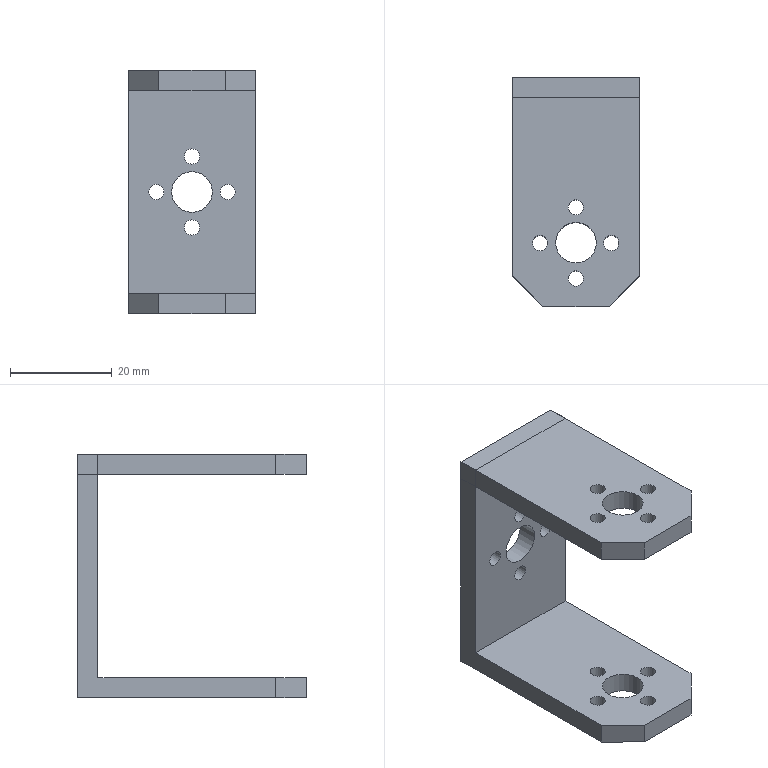Part | NX | features DATUM_CSYS 4, EXTRUDE 3, MOVE_FACE 3, SKETCH 3, EXTRACT_BODY 2, EXTRACT_FACE 2, EXTRACT_STRING 2, Instance Feature 1, Mirror Feature 1, Pattern Geometry 1 | 2 solids | 33 faces | box 25 x 45 x 48 mm | volume 12170 mm3 | plane 18 | cylinder 15 | commonest cylinder face diameters 3 x12 8 x3
STEP:
#1=CARTESIAN_POINT('',(-12.454,5.071,-2.));
#2=VERTEX_POINT('',#1);
#3=CARTESIAN_POINT('',(-12.454,44.071,-2.));
#4=VERTEX_POINT('',#3);
#5=CARTESIAN_POINT('',(-12.454,24.071,-2.));
#6=DIRECTION('',(0.,1.,0.));
#7=VECTOR('',#6,1000.);
#8=LINE('',#5,#7);
#9=EDGE_CURVE('',#2,#4,#8,.T.);
#10=ORIENTED_EDGE('',*,*,#9,.F.);
#11=CARTESIAN_POINT('',(-12.454,5.071,2.));
#12=VERTEX_POINT('',#11);
#13=CARTESIAN_POINT('',(-12.454,5.071,8.));
#14=DIRECTION('',(0.,0.,-1.));
#15=VECTOR('',#14,1000.);
#16=LINE('',#13,#15);
#17=EDGE_CURVE('',#12,#2,#16,.T.);
#18=ORIENTED_EDGE('',*,*,#17,.F.);
#19=CARTESIAN_POINT('',(-12.454,44.071,2.));
#20=VERTEX_POINT('',#19);
#21=CARTESIAN_POINT('',(-12.454,5.071,2.));
#22=DIRECTION('',(0.,1.,0.));
#23=VECTOR('',#22,1000.);
#24=LINE('',#21,#23);
#25=EDGE_CURVE('',#12,#20,#24,.T.);
#26=ORIENTED_EDGE('',*,*,#25,.T.);
#27=CARTESIAN_POINT('',(-12.454,44.071,8.));
#28=DIRECTION('',(0.,0.,-1.));
#29=VECTOR('',#28,1000.);
#30=LINE('',#27,#29);
#31=EDGE_CURVE('',#20,#4,#30,.T.);
#32=ORIENTED_EDGE('',*,*,#31,.T.);
#33=EDGE_LOOP('',(#10,#18,#26,#32));
#34=FACE_BOUND('',#33,.T.);
#35=CARTESIAN_POINT('',(-12.454,24.071,8.));
#36=DIRECTION('',(-1.,0.,0.));
#37=DIRECTION('',(0.,-1.,0.));
#38=AXIS2_PLACEMENT_3D('',#35,#36,#37);
#39=PLANE('',#38);
#40=ADVANCED_FACE('',(#34),#39,.T.);
#41=CARTESIAN_POINT('',(12.546,44.071,-2.));
#42=VERTEX_POINT('',#41);
#43=CARTESIAN_POINT('',(-12.454,44.071,-2.));
#44=DIRECTION('',(1.,0.,0.));
#45=VECTOR('',#44,1000.);
#46=LINE('',#43,#45);
#47=EDGE_CURVE('',#4,#42,#46,.T.);
#48=ORIENTED_EDGE('',*,*,#47,.F.);
#49=ORIENTED_EDGE('',*,*,#31,.F.);
#50=CARTESIAN_POINT('',(12.546,44.071,2.));
#51=VERTEX_POINT('',#50);
#52=CARTESIAN_POINT('',(-12.454,44.071,2.));
#53=DIRECTION('',(1.,0.,0.));
#54=VECTOR('',#53,1000.);
#55=LINE('',#52,#54);
#56=EDGE_CURVE('',#20,#51,#55,.T.);
#57=ORIENTED_EDGE('',*,*,#56,.T.);
#58=CARTESIAN_POINT('',(12.546,44.071,8.));
#59=DIRECTION('',(0.,0.,-1.));
#60=VECTOR('',#59,1000.);
#61=LINE('',#58,#60);
#62=EDGE_CURVE('',#51,#42,#61,.T.);
#63=ORIENTED_EDGE('',*,*,#62,.T.);
#64=EDGE_LOOP('',(#48,#49,#57,#63));
#65=FACE_BOUND('',#64,.T.);
#66=CARTESIAN_POINT('',(-12.454,44.071,8.));
#67=DIRECTION('',(0.,1.,0.));
#68=DIRECTION('',(0.,0.,1.));
#69=AXIS2_PLACEMENT_3D('',#66,#67,#68);
#70=PLANE('',#69);
#71=ADVANCED_FACE('',(#65),#70,.T.);
#72=CARTESIAN_POINT('',(12.546,5.071,-2.));
#73=VERTEX_POINT('',#72);
#74=CARTESIAN_POINT('',(12.546,24.071,-2.));
#75=DIRECTION('',(0.,-1.,0.));
#76=VECTOR('',#75,1000.);
#77=LINE('',#74,#76);
#78=EDGE_CURVE('',#42,#73,#77,.T.);
#79=ORIENTED_EDGE('',*,*,#78,.F.);
#80=ORIENTED_EDGE('',*,*,#62,.F.);
#81=CARTESIAN_POINT('',(12.546,5.071,2.));
#82=VERTEX_POINT('',#81);
#83=CARTESIAN_POINT('',(12.546,44.071,2.));
#84=DIRECTION('',(0.,-1.,0.));
#85=VECTOR('',#84,1000.);
#86=LINE('',#83,#85);
#87=EDGE_CURVE('',#51,#82,#86,.T.);
#88=ORIENTED_EDGE('',*,*,#87,.T.);
#89=CARTESIAN_POINT('',(12.546,5.071,8.));
#90=DIRECTION('',(0.,0.,-1.));
#91=VECTOR('',#90,1000.);
#92=LINE('',#89,#91);
#93=EDGE_CURVE('',#82,#73,#92,.T.);
#94=ORIENTED_EDGE('',*,*,#93,.T.);
#95=EDGE_LOOP('',(#79,#80,#88,#94));
#96=FACE_BOUND('',#95,.T.);
#97=CARTESIAN_POINT('',(12.546,24.071,8.));
#98=DIRECTION('',(1.,0.,0.));
#99=DIRECTION('',(0.,1.,0.));
#100=AXIS2_PLACEMENT_3D('',#97,#98,#99);
#101=PLANE('',#100);
#102=ADVANCED_FACE('',(#96),#101,.T.);
#103=CARTESIAN_POINT('',(6.546,-0.9291,-2.));
#104=VERTEX_POINT('',#103);
#105=CARTESIAN_POINT('',(12.546,5.071,-2.));
#106=DIRECTION('',(-0.7071,-0.7071,0.));
#107=VECTOR('',#106,1000.);
#108=LINE('',#105,#107);
#109=EDGE_CURVE('',#73,#104,#108,.T.);
#110=ORIENTED_EDGE('',*,*,#109,.F.);
#111=ORIENTED_EDGE('',*,*,#93,.F.);
#112=CARTESIAN_POINT('',(6.546,-0.9291,2.));
#113=VERTEX_POINT('',#112);
#114=CARTESIAN_POINT('',(12.546,5.071,2.));
#115=DIRECTION('',(-0.7071,-0.7071,0.));
#116=VECTOR('',#115,1000.);
#117=LINE('',#114,#116);
#118=EDGE_CURVE('',#82,#113,#117,.T.);
#119=ORIENTED_EDGE('',*,*,#118,.T.);
#120=CARTESIAN_POINT('',(6.546,-0.9291,8.));
#121=DIRECTION('',(0.,0.,-1.));
#122=VECTOR('',#121,1000.);
#123=LINE('',#120,#122);
#124=EDGE_CURVE('',#113,#104,#123,.T.);
#125=ORIENTED_EDGE('',*,*,#124,.T.);
#126=EDGE_LOOP('',(#110,#111,#119,#125));
#127=FACE_BOUND('',#126,.T.);
#128=CARTESIAN_POINT('',(12.546,5.071,8.));
#129=DIRECTION('',(0.7071,-0.7071,0.));
#130=DIRECTION('',(0.7071,0.7071,0.));
#131=AXIS2_PLACEMENT_3D('',#128,#129,#130);
#132=PLANE('',#131);
#133=ADVANCED_FACE('',(#127),#132,.T.);
#134=CARTESIAN_POINT('',(-6.454,-0.9291,-2.));
#135=VERTEX_POINT('',#134);
#136=CARTESIAN_POINT('',(6.546,-0.9291,-2.));
#137=DIRECTION('',(-1.,0.,0.));
#138=VECTOR('',#137,1000.);
#139=LINE('',#136,#138);
#140=EDGE_CURVE('',#104,#135,#139,.T.);
#141=ORIENTED_EDGE('',*,*,#140,.F.);
#142=ORIENTED_EDGE('',*,*,#124,.F.);
#143=CARTESIAN_POINT('',(-6.454,-0.9291,2.));
#144=VERTEX_POINT('',#143);
#145=CARTESIAN_POINT('',(6.546,-0.9291,2.));
#146=DIRECTION('',(-1.,0.,0.));
#147=VECTOR('',#146,1000.);
#148=LINE('',#145,#147);
#149=EDGE_CURVE('',#113,#144,#148,.T.);
#150=ORIENTED_EDGE('',*,*,#149,.T.);
#151=CARTESIAN_POINT('',(-6.454,-0.9291,8.));
#152=DIRECTION('',(0.,0.,-1.));
#153=VECTOR('',#152,1000.);
#154=LINE('',#151,#153);
#155=EDGE_CURVE('',#144,#135,#154,.T.);
#156=ORIENTED_EDGE('',*,*,#155,.T.);
#157=EDGE_LOOP('',(#141,#142,#150,#156));
#158=FACE_BOUND('',#157,.T.);
#159=CARTESIAN_POINT('',(6.546,-0.9291,8.));
#160=DIRECTION('',(0.,-1.,0.));
#161=DIRECTION('',(0.,0.,-1.));
#162=AXIS2_PLACEMENT_3D('',#159,#160,#161);
#163=PLANE('',#162);
#164=ADVANCED_FACE('',(#158),#163,.T.);
#165=CARTESIAN_POINT('',(1.5,4.5,2.));
#166=VERTEX_POINT('',#165);
#167=CARTESIAN_POINT('',(0.,4.5,2.));
#168=DIRECTION('',(0.,0.,-1.));
#169=DIRECTION('',(1.,0.,0.));
#170=AXIS2_PLACEMENT_3D('',#167,#168,#169);
#171=CIRCLE('',#170,1.5);
#172=EDGE_CURVE('',#166,#166,#171,.T.);
#173=ORIENTED_EDGE('',*,*,#172,.F.);
#174=EDGE_LOOP('',(#173));
#175=FACE_BOUND('',#174,.T.);
#176=CARTESIAN_POINT('',(1.5,4.5,-2.));
#177=VERTEX_POINT('',#176);
#178=CARTESIAN_POINT('',(0.,4.5,-2.));
#179=DIRECTION('',(0.,0.,-1.));
#180=DIRECTION('',(1.,0.,0.));
#181=AXIS2_PLACEMENT_3D('',#178,#179,#180);
#182=CIRCLE('',#181,1.5);
#183=EDGE_CURVE('',#177,#177,#182,.T.);
#184=ORIENTED_EDGE('',*,*,#183,.T.);
#185=EDGE_LOOP('',(#184));
#186=FACE_BOUND('',#185,.T.);
#187=CARTESIAN_POINT('',(0.,4.5,8.));
#188=DIRECTION('',(0.,0.,-1.));
#189=DIRECTION('',(-1.,0.,0.));
#190=AXIS2_PLACEMENT_3D('',#187,#188,#189);
#191=CYLINDRICAL_SURFACE('',#190,1.5);
#192=ADVANCED_FACE('',(#175,#186),#191,.F.);
#193=CARTESIAN_POINT('',(-5.5,11.5,2.));
#194=VERTEX_POINT('',#193);
#195=CARTESIAN_POINT('',(-7.,11.5,2.));
#196=DIRECTION('',(0.,0.,-1.));
#197=DIRECTION('',(1.,0.,0.));
#198=AXIS2_PLACEMENT_3D('',#195,#196,#197);
#199=CIRCLE('',#198,1.5);
#200=EDGE_CURVE('',#194,#194,#199,.T.);
#201=ORIENTED_EDGE('',*,*,#200,.F.);
#202=EDGE_LOOP('',(#201));
#203=FACE_BOUND('',#202,.T.);
#204=CARTESIAN_POINT('',(-5.5,11.5,-2.));
#205=VERTEX_POINT('',#204);
#206=CARTESIAN_POINT('',(-7.,11.5,-2.));
#207=DIRECTION('',(0.,0.,-1.));
#208=DIRECTION('',(1.,0.,0.));
#209=AXIS2_PLACEMENT_3D('',#206,#207,#208);
#210=CIRCLE('',#209,1.5);
#211=EDGE_CURVE('',#205,#205,#210,.T.);
#212=ORIENTED_EDGE('',*,*,#211,.T.);
#213=EDGE_LOOP('',(#212));
#214=FACE_BOUND('',#213,.T.);
#215=CARTESIAN_POINT('',(-7.,11.5,8.));
#216=DIRECTION('',(0.,0.,-1.));
#217=DIRECTION('',(-1.,0.,0.));
#218=AXIS2_PLACEMENT_3D('',#215,#216,#217);
#219=CYLINDRICAL_SURFACE('',#218,1.5);
#220=ADVANCED_FACE('',(#203,#214),#219,.F.);
#221=CARTESIAN_POINT('',(4.046,11.571,2.));
#222=VERTEX_POINT('',#221);
#223=CARTESIAN_POINT('',(0.04628,11.571,2.));
#224=DIRECTION('',(0.,0.,-1.));
#225=DIRECTION('',(1.,0.,0.));
#226=AXIS2_PLACEMENT_3D('',#223,#224,#225);
#227=CIRCLE('',#226,4.);
#228=EDGE_CURVE('',#222,#222,#227,.T.);
#229=ORIENTED_EDGE('',*,*,#228,.F.);
#230=EDGE_LOOP('',(#229));
#231=FACE_BOUND('',#230,.T.);
#232=CARTESIAN_POINT('',(4.046,11.571,-2.));
#233=VERTEX_POINT('',#232);
#234=CARTESIAN_POINT('',(0.04628,11.571,-2.));
#235=DIRECTION('',(0.,0.,-1.));
#236=DIRECTION('',(1.,0.,0.));
#237=AXIS2_PLACEMENT_3D('',#234,#235,#236);
#238=CIRCLE('',#237,4.);
#239=EDGE_CURVE('',#233,#233,#238,.T.);
#240=ORIENTED_EDGE('',*,*,#239,.T.);
#241=EDGE_LOOP('',(#240));
#242=FACE_BOUND('',#241,.T.);
#243=CARTESIAN_POINT('',(0.04628,11.571,8.));
#244=DIRECTION('',(0.,0.,-1.));
#245=DIRECTION('',(-1.,0.,0.));
#246=AXIS2_PLACEMENT_3D('',#243,#244,#245);
#247=CYLINDRICAL_SURFACE('',#246,4.);
#248=ADVANCED_FACE('',(#231,#242),#247,.F.);
#249=CARTESIAN_POINT('',(1.5,18.5,2.));
#250=VERTEX_POINT('',#249);
#251=CARTESIAN_POINT('',(0.,18.5,2.));
#252=DIRECTION('',(0.,0.,-1.));
#253=DIRECTION('',(1.,0.,0.));
#254=AXIS2_PLACEMENT_3D('',#251,#252,#253);
#255=CIRCLE('',#254,1.5);
#256=EDGE_CURVE('',#250,#250,#255,.T.);
#257=ORIENTED_EDGE('',*,*,#256,.F.);
#258=EDGE_LOOP('',(#257));
#259=FACE_BOUND('',#258,.T.);
#260=CARTESIAN_POINT('',(1.5,18.5,-2.));
#261=VERTEX_POINT('',#260);
#262=CARTESIAN_POINT('',(0.,18.5,-2.));
#263=DIRECTION('',(0.,0.,-1.));
#264=DIRECTION('',(1.,0.,0.));
#265=AXIS2_PLACEMENT_3D('',#262,#263,#264);
#266=CIRCLE('',#265,1.5);
#267=EDGE_CURVE('',#261,#261,#266,.T.);
#268=ORIENTED_EDGE('',*,*,#267,.T.);
#269=EDGE_LOOP('',(#268));
#270=FACE_BOUND('',#269,.T.);
#271=CARTESIAN_POINT('',(0.,18.5,8.));
#272=DIRECTION('',(0.,0.,-1.));
#273=DIRECTION('',(-1.,0.,0.));
#274=AXIS2_PLACEMENT_3D('',#271,#272,#273);
#275=CYLINDRICAL_SURFACE('',#274,1.5);
#276=ADVANCED_FACE('',(#259,#270),#275,.F.);
#277=CARTESIAN_POINT('',(-6.454,-0.9291,-2.));
#278=DIRECTION('',(-0.7071,0.7071,0.));
#279=VECTOR('',#278,1000.);
#280=LINE('',#277,#279);
#281=EDGE_CURVE('',#135,#2,#280,.T.);
#282=ORIENTED_EDGE('',*,*,#281,.F.);
#283=ORIENTED_EDGE('',*,*,#155,.F.);
#284=CARTESIAN_POINT('',(-6.454,-0.9291,2.));
#285=DIRECTION('',(-0.7071,0.7071,0.));
#286=VECTOR('',#285,1000.);
#287=LINE('',#284,#286);
#288=EDGE_CURVE('',#144,#12,#287,.T.);
#289=ORIENTED_EDGE('',*,*,#288,.T.);
#290=ORIENTED_EDGE('',*,*,#17,.T.);
#291=EDGE_LOOP('',(#282,#283,#289,#290));
#292=FACE_BOUND('',#291,.T.);
#293=CARTESIAN_POINT('',(-6.454,-0.9291,8.));
#294=DIRECTION('',(-0.7071,-0.7071,0.));
#295=DIRECTION('',(0.7071,-0.7071,0.));
#296=AXIS2_PLACEMENT_3D('',#293,#294,#295);
#297=PLANE('',#296);
#298=ADVANCED_FACE('',(#292),#297,.T.);
#299=CARTESIAN_POINT('',(8.5,11.5,2.));
#300=VERTEX_POINT('',#299);
#301=CARTESIAN_POINT('',(7.,11.5,2.));
#302=DIRECTION('',(0.,0.,-1.));
#303=DIRECTION('',(1.,0.,0.));
#304=AXIS2_PLACEMENT_3D('',#301,#302,#303);
#305=CIRCLE('',#304,1.5);
#306=EDGE_CURVE('',#300,#300,#305,.T.);
#307=ORIENTED_EDGE('',*,*,#306,.F.);
#308=EDGE_LOOP('',(#307));
#309=FACE_BOUND('',#308,.T.);
#310=CARTESIAN_POINT('',(8.5,11.5,-2.));
#311=VERTEX_POINT('',#310);
#312=CARTESIAN_POINT('',(7.,11.5,-2.));
#313=DIRECTION('',(0.,0.,-1.));
#314=DIRECTION('',(1.,0.,0.));
#315=AXIS2_PLACEMENT_3D('',#312,#313,#314);
#316=CIRCLE('',#315,1.5);
#317=EDGE_CURVE('',#311,#311,#316,.T.);
#318=ORIENTED_EDGE('',*,*,#317,.T.);
#319=EDGE_LOOP('',(#318));
#320=FACE_BOUND('',#319,.T.);
#321=CARTESIAN_POINT('',(7.,11.5,8.));
#322=DIRECTION('',(0.,0.,-1.));
#323=DIRECTION('',(-1.,0.,0.));
#324=AXIS2_PLACEMENT_3D('',#321,#322,#323);
#325=CYLINDRICAL_SURFACE('',#324,1.5);
#326=ADVANCED_FACE('',(#309,#320),#325,.F.);
#327=ORIENTED_EDGE('',*,*,#25,.F.);
#328=ORIENTED_EDGE('',*,*,#288,.F.);
#329=ORIENTED_EDGE('',*,*,#149,.F.);
#330=ORIENTED_EDGE('',*,*,#118,.F.);
#331=ORIENTED_EDGE('',*,*,#87,.F.);
#332=ORIENTED_EDGE('',*,*,#56,.F.);
#333=EDGE_LOOP('',(#327,#328,#329,#330,#331,#332));
#334=FACE_BOUND('',#333,.T.);
#335=ORIENTED_EDGE('',*,*,#256,.T.);
#336=EDGE_LOOP('',(#335));
#337=FACE_BOUND('',#336,.T.);
#338=ORIENTED_EDGE('',*,*,#228,.T.);
#339=EDGE_LOOP('',(#338));
#340=FACE_BOUND('',#339,.T.);
#341=ORIENTED_EDGE('',*,*,#200,.T.);
#342=EDGE_LOOP('',(#341));
#343=FACE_BOUND('',#342,.T.);
#344=ORIENTED_EDGE('',*,*,#172,.T.);
#345=EDGE_LOOP('',(#344));
#346=FACE_BOUND('',#345,.T.);
#347=ORIENTED_EDGE('',*,*,#306,.T.);
#348=EDGE_LOOP('',(#347));
#349=FACE_BOUND('',#348,.T.);
#350=CARTESIAN_POINT('',(0.,18.5,2.));
#351=DIRECTION('',(0.,0.,-1.));
#352=DIRECTION('',(-1.,0.,0.));
#353=AXIS2_PLACEMENT_3D('',#350,#351,#352);
#354=PLANE('',#353);
#355=ADVANCED_FACE('',(#334,#337,#340,#343,#346,#349),#354,.F.);
#356=ORIENTED_EDGE('',*,*,#281,.T.);
#357=ORIENTED_EDGE('',*,*,#9,.T.);
#358=ORIENTED_EDGE('',*,*,#47,.T.);
#359=ORIENTED_EDGE('',*,*,#78,.T.);
#360=ORIENTED_EDGE('',*,*,#109,.T.);
#361=ORIENTED_EDGE('',*,*,#140,.T.);
#362=EDGE_LOOP('',(#356,#357,#358,#359,#360,#361));
#363=FACE_BOUND('',#362,.T.);
#364=ORIENTED_EDGE('',*,*,#267,.F.);
#365=EDGE_LOOP('',(#364));
#366=FACE_BOUND('',#365,.T.);
#367=ORIENTED_EDGE('',*,*,#239,.F.);
#368=EDGE_LOOP('',(#367));
#369=FACE_BOUND('',#368,.T.);
#370=ORIENTED_EDGE('',*,*,#211,.F.);
#371=EDGE_LOOP('',(#370));
#372=FACE_BOUND('',#371,.T.);
#373=ORIENTED_EDGE('',*,*,#183,.F.);
#374=EDGE_LOOP('',(#373));
#375=FACE_BOUND('',#374,.T.);
#376=ORIENTED_EDGE('',*,*,#317,.F.);
#377=EDGE_LOOP('',(#376));
#378=FACE_BOUND('',#377,.T.);
#379=CARTESIAN_POINT('',(0.,18.5,-2.));
#380=DIRECTION('',(0.,0.,-1.));
#381=DIRECTION('',(-1.,0.,0.));
#382=AXIS2_PLACEMENT_3D('',#379,#380,#381);
#383=PLANE('',#382);
#384=ADVANCED_FACE('',(#363,#366,#369,#372,#375,#378),#383,.T.);
#385=CLOSED_SHELL('',(#40,#71,#102,#133,#164,#192,#220,#248,#276,#298,#326,#355,#384));
#386=MANIFOLD_SOLID_BREP('',#385);
#387=CARTESIAN_POINT('',(8.5,11.5,-42.));
#388=VERTEX_POINT('',#387);
#389=CARTESIAN_POINT('',(7.,11.5,-42.));
#390=DIRECTION('',(0.,0.,-1.));
#391=DIRECTION('',(1.,0.,0.));
#392=AXIS2_PLACEMENT_3D('',#389,#390,#391);
#393=CIRCLE('',#392,1.5);
#394=EDGE_CURVE('',#388,#388,#393,.T.);
#395=ORIENTED_EDGE('',*,*,#394,.T.);
#396=EDGE_LOOP('',(#395));
#397=FACE_BOUND('',#396,.T.);
#398=CARTESIAN_POINT('',(1.5,4.5,-42.));
#399=VERTEX_POINT('',#398);
#400=CARTESIAN_POINT('',(0.,4.5,-42.));
#401=DIRECTION('',(0.,0.,-1.));
#402=DIRECTION('',(1.,0.,0.));
#403=AXIS2_PLACEMENT_3D('',#400,#401,#402);
#404=CIRCLE('',#403,1.5);
#405=EDGE_CURVE('',#399,#399,#404,.T.);
#406=ORIENTED_EDGE('',*,*,#405,.T.);
#407=EDGE_LOOP('',(#406));
#408=FACE_BOUND('',#407,.T.);
#409=CARTESIAN_POINT('',(-5.5,11.5,-42.));
#410=VERTEX_POINT('',#409);
#411=CARTESIAN_POINT('',(-7.,11.5,-42.));
#412=DIRECTION('',(0.,0.,-1.));
#413=DIRECTION('',(1.,0.,0.));
#414=AXIS2_PLACEMENT_3D('',#411,#412,#413);
#415=CIRCLE('',#414,1.5);
#416=EDGE_CURVE('',#410,#410,#415,.T.);
#417=ORIENTED_EDGE('',*,*,#416,.T.);
#418=EDGE_LOOP('',(#417));
#419=FACE_BOUND('',#418,.T.);
#420=CARTESIAN_POINT('',(4.046,11.571,-42.));
#421=VERTEX_POINT('',#420);
#422=CARTESIAN_POINT('',(0.04628,11.571,-42.));
#423=DIRECTION('',(0.,0.,-1.));
#424=DIRECTION('',(1.,0.,0.));
#425=AXIS2_PLACEMENT_3D('',#422,#423,#424);
#426=CIRCLE('',#425,4.);
#427=EDGE_CURVE('',#421,#421,#426,.T.);
#428=ORIENTED_EDGE('',*,*,#427,.T.);
#429=EDGE_LOOP('',(#428));
#430=FACE_BOUND('',#429,.T.);
#431=CARTESIAN_POINT('',(1.5,18.5,-42.));
#432=VERTEX_POINT('',#431);
#433=CARTESIAN_POINT('',(0.,18.5,-42.));
#434=DIRECTION('',(0.,0.,-1.));
#435=DIRECTION('',(1.,0.,0.));
#436=AXIS2_PLACEMENT_3D('',#433,#434,#435);
#437=CIRCLE('',#436,1.5);
#438=EDGE_CURVE('',#432,#432,#437,.T.);
#439=ORIENTED_EDGE('',*,*,#438,.T.);
#440=EDGE_LOOP('',(#439));
#441=FACE_BOUND('',#440,.T.);
#442=CARTESIAN_POINT('',(12.546,40.071,-42.));
#443=VERTEX_POINT('',#442);
#444=CARTESIAN_POINT('',(-12.454,40.071,-42.));
#445=VERTEX_POINT('',#444);
#446=CARTESIAN_POINT('',(0.,40.071,-42.));
#447=DIRECTION('',(1.,0.,0.));
#448=VECTOR('',#447,1000.);
#449=LINE('',#446,#448);
#450=EDGE_CURVE('',#443,#445,#449,.F.);
#451=ORIENTED_EDGE('',*,*,#450,.T.);
#452=CARTESIAN_POINT('',(-12.454,5.071,-42.));
#453=VERTEX_POINT('',#452);
#454=CARTESIAN_POINT('',(-12.454,24.071,-42.));
#455=DIRECTION('',(0.,1.,0.));
#456=VECTOR('',#455,1000.);
#457=LINE('',#454,#456);
#458=EDGE_CURVE('',#453,#445,#457,.T.);
#459=ORIENTED_EDGE('',*,*,#458,.F.);
#460=CARTESIAN_POINT('',(-6.454,-0.9291,-42.));
#461=VERTEX_POINT('',#460);
#462=CARTESIAN_POINT('',(-6.454,-0.9291,-42.));
#463=DIRECTION('',(-0.7071,0.7071,0.));
#464=VECTOR('',#463,1000.);
#465=LINE('',#462,#464);
#466=EDGE_CURVE('',#461,#453,#465,.T.);
#467=ORIENTED_EDGE('',*,*,#466,.F.);
#468=CARTESIAN_POINT('',(6.546,-0.9291,-42.));
#469=VERTEX_POINT('',#468);
#470=CARTESIAN_POINT('',(6.546,-0.9291,-42.));
#471=DIRECTION('',(-1.,0.,0.));
#472=VECTOR('',#471,1000.);
#473=LINE('',#470,#472);
#474=EDGE_CURVE('',#469,#461,#473,.T.);
#475=ORIENTED_EDGE('',*,*,#474,.F.);
#476=CARTESIAN_POINT('',(12.546,5.071,-42.));
#477=VERTEX_POINT('',#476);
#478=CARTESIAN_POINT('',(12.546,5.071,-42.));
#479=DIRECTION('',(-0.7071,-0.7071,0.));
#480=VECTOR('',#479,1000.);
#481=LINE('',#478,#480);
#482=EDGE_CURVE('',#477,#469,#481,.T.);
#483=ORIENTED_EDGE('',*,*,#482,.F.);
#484=CARTESIAN_POINT('',(12.546,24.071,-42.));
#485=DIRECTION('',(0.,-1.,0.));
#486=VECTOR('',#485,1000.);
#487=LINE('',#484,#486);
#488=EDGE_CURVE('',#443,#477,#487,.T.);
#489=ORIENTED_EDGE('',*,*,#488,.F.);
#490=EDGE_LOOP('',(#451,#459,#467,#475,#483,#489));
#491=FACE_BOUND('',#490,.T.);
#492=CARTESIAN_POINT('',(0.,18.5,-42.));
#493=DIRECTION('',(0.,0.,-1.));
#494=DIRECTION('',(-1.,0.,0.));
#495=AXIS2_PLACEMENT_3D('',#492,#493,#494);
#496=PLANE('',#495);
#497=ADVANCED_FACE('',(#397,#408,#419,#430,#441,#491),#496,.F.);
#498=ORIENTED_EDGE('',*,*,#458,.T.);
#499=CARTESIAN_POINT('',(-12.454,40.071,2.));
#500=VERTEX_POINT('',#499);
#501=CARTESIAN_POINT('',(-12.454,40.071,4.));
#502=DIRECTION('',(0.,0.,-1.));
#503=VECTOR('',#502,1000.);
#504=LINE('',#501,#503);
#505=EDGE_CURVE('',#500,#445,#504,.T.);
#506=ORIENTED_EDGE('',*,*,#505,.F.);
#507=CARTESIAN_POINT('',(-12.454,44.071,2.));
#508=VERTEX_POINT('',#507);
#509=CARTESIAN_POINT('',(-12.454,40.071,2.));
#510=DIRECTION('',(0.,1.,0.));
#511=VECTOR('',#510,1000.);
#512=LINE('',#509,#511);
#513=EDGE_CURVE('',#500,#508,#512,.T.);
#514=ORIENTED_EDGE('',*,*,#513,.T.);
#515=CARTESIAN_POINT('',(-12.454,44.071,-46.));
#516=VERTEX_POINT('',#515);
#517=CARTESIAN_POINT('',(-12.454,44.071,-52.));
#518=DIRECTION('',(0.,0.,1.));
#519=VECTOR('',#518,1000.);
#520=LINE('',#517,#519);
#521=EDGE_CURVE('',#516,#508,#520,.T.);
#522=ORIENTED_EDGE('',*,*,#521,.F.);
#523=CARTESIAN_POINT('',(-12.454,5.071,-46.));
#524=VERTEX_POINT('',#523);
#525=CARTESIAN_POINT('',(-12.454,5.071,-46.));
#526=DIRECTION('',(0.,1.,0.));
#527=VECTOR('',#526,1000.);
#528=LINE('',#525,#527);
#529=EDGE_CURVE('',#524,#516,#528,.T.);
#530=ORIENTED_EDGE('',*,*,#529,.F.);
#531=CARTESIAN_POINT('',(-12.454,5.071,-52.));
#532=DIRECTION('',(0.,0.,1.));
#533=VECTOR('',#532,1000.);
#534=LINE('',#531,#533);
#535=EDGE_CURVE('',#524,#453,#534,.T.);
#536=ORIENTED_EDGE('',*,*,#535,.T.);
#537=EDGE_LOOP('',(#498,#506,#514,#522,#530,#536));
#538=FACE_BOUND('',#537,.T.);
#539=CARTESIAN_POINT('',(-12.454,24.071,-52.));
#540=DIRECTION('',(1.,0.,0.));
#541=DIRECTION('',(0.,1.,0.));
#542=AXIS2_PLACEMENT_3D('',#539,#540,#541);
#543=PLANE('',#542);
#544=ADVANCED_FACE('',(#538),#543,.F.);
#545=ORIENTED_EDGE('',*,*,#521,.T.);
#546=CARTESIAN_POINT('',(12.546,44.071,2.));
#547=VERTEX_POINT('',#546);
#548=CARTESIAN_POINT('',(12.546,44.071,2.));
#549=DIRECTION('',(-1.,0.,0.));
#550=VECTOR('',#549,1000.);
#551=LINE('',#548,#550);
#552=EDGE_CURVE('',#547,#508,#551,.T.);
#553=ORIENTED_EDGE('',*,*,#552,.F.);
#554=CARTESIAN_POINT('',(12.546,44.071,-46.));
#555=VERTEX_POINT('',#554);
#556=CARTESIAN_POINT('',(12.546,44.071,-52.));
#557=DIRECTION('',(0.,0.,1.));
#558=VECTOR('',#557,1000.);
#559=LINE('',#556,#558);
#560=EDGE_CURVE('',#555,#547,#559,.T.);
#561=ORIENTED_EDGE('',*,*,#560,.F.);
#562=CARTESIAN_POINT('',(-12.454,44.071,-46.));
#563=DIRECTION('',(1.,0.,0.));
#564=VECTOR('',#563,1000.);
#565=LINE('',#562,#564);
#566=EDGE_CURVE('',#516,#555,#565,.T.);
#567=ORIENTED_EDGE('',*,*,#566,.F.);
#568=EDGE_LOOP('',(#545,#553,#561,#567));
#569=FACE_BOUND('',#568,.T.);
#570=CARTESIAN_POINT('',(-6.954,44.071,-23.5));
#571=VERTEX_POINT('',#570);
#572=CARTESIAN_POINT('',(-6.954,44.071,-22.));
#573=DIRECTION('',(0.,1.,0.));
#574=DIRECTION('',(0.,0.,-1.));
#575=AXIS2_PLACEMENT_3D('',#572,#573,#574);
#576=CIRCLE('',#575,1.5);
#577=EDGE_CURVE('',#571,#571,#576,.T.);
#578=ORIENTED_EDGE('',*,*,#577,.F.);
#579=EDGE_LOOP('',(#578));
#580=FACE_BOUND('',#579,.T.);
#581=CARTESIAN_POINT('',(0.04628,44.071,-26.));
#582=VERTEX_POINT('',#581);
#583=CARTESIAN_POINT('',(0.04628,44.071,-22.));
#584=DIRECTION('',(0.,1.,0.));
#585=DIRECTION('',(0.,0.,-1.));
#586=AXIS2_PLACEMENT_3D('',#583,#584,#585);
#587=CIRCLE('',#586,4.);
#588=EDGE_CURVE('',#582,#582,#587,.T.);
#589=ORIENTED_EDGE('',*,*,#588,.F.);
#590=EDGE_LOOP('',(#589));
#591=FACE_BOUND('',#590,.T.);
#592=CARTESIAN_POINT('',(0.04628,44.071,-30.5));
#593=VERTEX_POINT('',#592);
#594=CARTESIAN_POINT('',(0.04628,44.071,-29.));
#595=DIRECTION('',(0.,1.,0.));
#596=DIRECTION('',(0.,0.,-1.));
#597=AXIS2_PLACEMENT_3D('',#594,#595,#596);
#598=CIRCLE('',#597,1.5);
#599=EDGE_CURVE('',#593,#593,#598,.T.);
#600=ORIENTED_EDGE('',*,*,#599,.F.);
#601=EDGE_LOOP('',(#600));
#602=FACE_BOUND('',#601,.T.);
#603=CARTESIAN_POINT('',(0.04628,44.071,-16.5));
#604=VERTEX_POINT('',#603);
#605=CARTESIAN_POINT('',(0.04628,44.071,-15.));
#606=DIRECTION('',(0.,1.,0.));
#607=DIRECTION('',(0.,0.,-1.));
#608=AXIS2_PLACEMENT_3D('',#605,#606,#607);
#609=CIRCLE('',#608,1.5);
#610=EDGE_CURVE('',#604,#604,#609,.T.);
#611=ORIENTED_EDGE('',*,*,#610,.F.);
#612=EDGE_LOOP('',(#611));
#613=FACE_BOUND('',#612,.T.);
#614=CARTESIAN_POINT('',(7.046,44.071,-23.5));
#615=VERTEX_POINT('',#614);
#616=CARTESIAN_POINT('',(7.046,44.071,-22.));
#617=DIRECTION('',(0.,1.,0.));
#618=DIRECTION('',(0.,0.,-1.));
#619=AXIS2_PLACEMENT_3D('',#616,#617,#618);
#620=CIRCLE('',#619,1.5);
#621=EDGE_CURVE('',#615,#615,#620,.T.);
#622=ORIENTED_EDGE('',*,*,#621,.F.);
#623=EDGE_LOOP('',(#622));
#624=FACE_BOUND('',#623,.T.);
#625=CARTESIAN_POINT('',(-12.454,44.071,-52.));
#626=DIRECTION('',(0.,-1.,0.));
#627=DIRECTION('',(0.,0.,-1.));
#628=AXIS2_PLACEMENT_3D('',#625,#626,#627);
#629=PLANE('',#628);
#630=ADVANCED_FACE('',(#569,#580,#591,#602,#613,#624),#629,.F.);
#631=CARTESIAN_POINT('',(12.546,5.071,-46.));
#632=VERTEX_POINT('',#631);
#633=CARTESIAN_POINT('',(12.546,5.071,-52.));
#634=DIRECTION('',(0.,0.,1.));
#635=VECTOR('',#634,1000.);
#636=LINE('',#633,#635);
#637=EDGE_CURVE('',#632,#477,#636,.T.);
#638=ORIENTED_EDGE('',*,*,#637,.F.);
#639=CARTESIAN_POINT('',(12.546,44.071,-46.));
#640=DIRECTION('',(0.,-1.,0.));
#641=VECTOR('',#640,1000.);
#642=LINE('',#639,#641);
#643=EDGE_CURVE('',#555,#632,#642,.T.);
#644=ORIENTED_EDGE('',*,*,#643,.F.);
#645=ORIENTED_EDGE('',*,*,#560,.T.);
#646=CARTESIAN_POINT('',(12.546,40.071,2.));
#647=VERTEX_POINT('',#646);
#648=CARTESIAN_POINT('',(12.546,40.071,2.));
#649=DIRECTION('',(0.,1.,0.));
#650=VECTOR('',#649,1000.);
#651=LINE('',#648,#650);
#652=EDGE_CURVE('',#647,#547,#651,.T.);
#653=ORIENTED_EDGE('',*,*,#652,.F.);
#654=CARTESIAN_POINT('',(12.546,40.071,-52.));
#655=DIRECTION('',(0.,0.,1.));
#656=VECTOR('',#655,1000.);
#657=LINE('',#654,#656);
#658=EDGE_CURVE('',#443,#647,#657,.T.);
#659=ORIENTED_EDGE('',*,*,#658,.F.);
#660=ORIENTED_EDGE('',*,*,#488,.T.);
#661=EDGE_LOOP('',(#638,#644,#645,#653,#659,#660));
#662=FACE_BOUND('',#661,.T.);
#663=CARTESIAN_POINT('',(12.546,24.071,-52.));
#664=DIRECTION('',(-1.,0.,0.));
#665=DIRECTION('',(0.,-1.,0.));
#666=AXIS2_PLACEMENT_3D('',#663,#664,#665);
#667=PLANE('',#666);
#668=ADVANCED_FACE('',(#662),#667,.F.);
#669=ORIENTED_EDGE('',*,*,#482,.T.);
#670=CARTESIAN_POINT('',(6.546,-0.9291,-46.));
#671=VERTEX_POINT('',#670);
#672=CARTESIAN_POINT('',(6.546,-0.9291,-52.));
#673=DIRECTION('',(0.,0.,1.));
#674=VECTOR('',#673,1000.);
#675=LINE('',#672,#674);
#676=EDGE_CURVE('',#671,#469,#675,.T.);
#677=ORIENTED_EDGE('',*,*,#676,.F.);
#678=CARTESIAN_POINT('',(12.546,5.071,-46.));
#679=DIRECTION('',(-0.7071,-0.7071,0.));
#680=VECTOR('',#679,1000.);
#681=LINE('',#678,#680);
#682=EDGE_CURVE('',#632,#671,#681,.T.);
#683=ORIENTED_EDGE('',*,*,#682,.F.);
#684=ORIENTED_EDGE('',*,*,#637,.T.);
#685=EDGE_LOOP('',(#669,#677,#683,#684));
#686=FACE_BOUND('',#685,.T.);
#687=CARTESIAN_POINT('',(12.546,5.071,-52.));
#688=DIRECTION('',(-0.7071,0.7071,0.));
#689=DIRECTION('',(-0.7071,-0.7071,0.));
#690=AXIS2_PLACEMENT_3D('',#687,#688,#689);
#691=PLANE('',#690);
#692=ADVANCED_FACE('',(#686),#691,.F.);
#693=ORIENTED_EDGE('',*,*,#474,.T.);
#694=CARTESIAN_POINT('',(-6.454,-0.9291,-46.));
#695=VERTEX_POINT('',#694);
#696=CARTESIAN_POINT('',(-6.454,-0.9291,-52.));
#697=DIRECTION('',(0.,0.,1.));
#698=VECTOR('',#697,1000.);
#699=LINE('',#696,#698);
#700=EDGE_CURVE('',#695,#461,#699,.T.);
#701=ORIENTED_EDGE('',*,*,#700,.F.);
#702=CARTESIAN_POINT('',(6.546,-0.9291,-46.));
#703=DIRECTION('',(-1.,0.,0.));
#704=VECTOR('',#703,1000.);
#705=LINE('',#702,#704);
#706=EDGE_CURVE('',#671,#695,#705,.T.);
#707=ORIENTED_EDGE('',*,*,#706,.F.);
#708=ORIENTED_EDGE('',*,*,#676,.T.);
#709=EDGE_LOOP('',(#693,#701,#707,#708));
#710=FACE_BOUND('',#709,.T.);
#711=CARTESIAN_POINT('',(6.546,-0.9291,-52.));
#712=DIRECTION('',(0.,1.,0.));
#713=DIRECTION('',(0.,0.,1.));
#714=AXIS2_PLACEMENT_3D('',#711,#712,#713);
#715=PLANE('',#714);
#716=ADVANCED_FACE('',(#710),#715,.F.);
#717=CARTESIAN_POINT('',(1.5,4.5,-46.));
#718=VERTEX_POINT('',#717);
#719=CARTESIAN_POINT('',(0.,4.5,-46.));
#720=DIRECTION('',(0.,0.,-1.));
#721=DIRECTION('',(1.,0.,0.));
#722=AXIS2_PLACEMENT_3D('',#719,#720,#721);
#723=CIRCLE('',#722,1.5);
#724=EDGE_CURVE('',#718,#718,#723,.T.);
#725=ORIENTED_EDGE('',*,*,#724,.T.);
#726=EDGE_LOOP('',(#725));
#727=FACE_BOUND('',#726,.T.);
#728=ORIENTED_EDGE('',*,*,#405,.F.);
#729=EDGE_LOOP('',(#728));
#730=FACE_BOUND('',#729,.T.);
#731=CARTESIAN_POINT('',(0.,4.5,-52.));
#732=DIRECTION('',(0.,0.,1.));
#733=DIRECTION('',(1.,0.,0.));
#734=AXIS2_PLACEMENT_3D('',#731,#732,#733);
#735=CYLINDRICAL_SURFACE('',#734,1.5);
#736=ADVANCED_FACE('',(#727,#730),#735,.F.);
#737=CARTESIAN_POINT('',(-5.5,11.5,-46.));
#738=VERTEX_POINT('',#737);
#739=CARTESIAN_POINT('',(-7.,11.5,-46.));
#740=DIRECTION('',(0.,0.,-1.));
#741=DIRECTION('',(1.,0.,0.));
#742=AXIS2_PLACEMENT_3D('',#739,#740,#741);
#743=CIRCLE('',#742,1.5);
#744=EDGE_CURVE('',#738,#738,#743,.T.);
#745=ORIENTED_EDGE('',*,*,#744,.T.);
#746=EDGE_LOOP('',(#745));
#747=FACE_BOUND('',#746,.T.);
#748=ORIENTED_EDGE('',*,*,#416,.F.);
#749=EDGE_LOOP('',(#748));
#750=FACE_BOUND('',#749,.T.);
#751=CARTESIAN_POINT('',(-7.,11.5,-52.));
#752=DIRECTION('',(0.,0.,1.));
#753=DIRECTION('',(1.,0.,0.));
#754=AXIS2_PLACEMENT_3D('',#751,#752,#753);
#755=CYLINDRICAL_SURFACE('',#754,1.5);
#756=ADVANCED_FACE('',(#747,#750),#755,.F.);
#757=CARTESIAN_POINT('',(4.046,11.571,-46.));
#758=VERTEX_POINT('',#757);
#759=CARTESIAN_POINT('',(0.04628,11.571,-46.));
#760=DIRECTION('',(0.,0.,-1.));
#761=DIRECTION('',(1.,0.,0.));
#762=AXIS2_PLACEMENT_3D('',#759,#760,#761);
#763=CIRCLE('',#762,4.);
#764=EDGE_CURVE('',#758,#758,#763,.T.);
#765=ORIENTED_EDGE('',*,*,#764,.T.);
#766=EDGE_LOOP('',(#765));
#767=FACE_BOUND('',#766,.T.);
#768=ORIENTED_EDGE('',*,*,#427,.F.);
#769=EDGE_LOOP('',(#768));
#770=FACE_BOUND('',#769,.T.);
#771=CARTESIAN_POINT('',(0.04628,11.571,-52.));
#772=DIRECTION('',(0.,0.,1.));
#773=DIRECTION('',(1.,0.,0.));
#774=AXIS2_PLACEMENT_3D('',#771,#772,#773);
#775=CYLINDRICAL_SURFACE('',#774,4.);
#776=ADVANCED_FACE('',(#767,#770),#775,.F.);
#777=CARTESIAN_POINT('',(1.5,18.5,-46.));
#778=VERTEX_POINT('',#777);
#779=CARTESIAN_POINT('',(0.,18.5,-46.));
#780=DIRECTION('',(0.,0.,-1.));
#781=DIRECTION('',(1.,0.,0.));
#782=AXIS2_PLACEMENT_3D('',#779,#780,#781);
#783=CIRCLE('',#782,1.5);
#784=EDGE_CURVE('',#778,#778,#783,.T.);
#785=ORIENTED_EDGE('',*,*,#784,.T.);
#786=EDGE_LOOP('',(#785));
#787=FACE_BOUND('',#786,.T.);
#788=ORIENTED_EDGE('',*,*,#438,.F.);
#789=EDGE_LOOP('',(#788));
#790=FACE_BOUND('',#789,.T.);
#791=CARTESIAN_POINT('',(0.,18.5,-52.));
#792=DIRECTION('',(0.,0.,1.));
#793=DIRECTION('',(1.,0.,0.));
#794=AXIS2_PLACEMENT_3D('',#791,#792,#793);
#795=CYLINDRICAL_SURFACE('',#794,1.5);
#796=ADVANCED_FACE('',(#787,#790),#795,.F.);
#797=ORIENTED_EDGE('',*,*,#466,.T.);
#798=ORIENTED_EDGE('',*,*,#535,.F.);
#799=CARTESIAN_POINT('',(-6.454,-0.9291,-46.));
#800=DIRECTION('',(-0.7071,0.7071,0.));
#801=VECTOR('',#800,1000.);
#802=LINE('',#799,#801);
#803=EDGE_CURVE('',#695,#524,#802,.T.);
#804=ORIENTED_EDGE('',*,*,#803,.F.);
#805=ORIENTED_EDGE('',*,*,#700,.T.);
#806=EDGE_LOOP('',(#797,#798,#804,#805));
#807=FACE_BOUND('',#806,.T.);
#808=CARTESIAN_POINT('',(-6.454,-0.9291,-52.));
#809=DIRECTION('',(0.7071,0.7071,0.));
#810=DIRECTION('',(-0.7071,0.7071,0.));
#811=AXIS2_PLACEMENT_3D('',#808,#809,#810);
#812=PLANE('',#811);
#813=ADVANCED_FACE('',(#807),#812,.F.);
#814=CARTESIAN_POINT('',(8.5,11.5,-46.));
#815=VERTEX_POINT('',#814);
#816=CARTESIAN_POINT('',(7.,11.5,-46.));
#817=DIRECTION('',(0.,0.,-1.));
#818=DIRECTION('',(1.,0.,0.));
#819=AXIS2_PLACEMENT_3D('',#816,#817,#818);
#820=CIRCLE('',#819,1.5);
#821=EDGE_CURVE('',#815,#815,#820,.T.);
#822=ORIENTED_EDGE('',*,*,#821,.T.);
#823=EDGE_LOOP('',(#822));
#824=FACE_BOUND('',#823,.T.);
#825=ORIENTED_EDGE('',*,*,#394,.F.);
#826=EDGE_LOOP('',(#825));
#827=FACE_BOUND('',#826,.T.);
#828=CARTESIAN_POINT('',(7.,11.5,-52.));
#829=DIRECTION('',(0.,0.,1.));
#830=DIRECTION('',(1.,0.,0.));
#831=AXIS2_PLACEMENT_3D('',#828,#829,#830);
#832=CYLINDRICAL_SURFACE('',#831,1.5);
#833=ADVANCED_FACE('',(#824,#827),#832,.F.);
#834=ORIENTED_EDGE('',*,*,#643,.T.);
#835=ORIENTED_EDGE('',*,*,#682,.T.);
#836=ORIENTED_EDGE('',*,*,#706,.T.);
#837=ORIENTED_EDGE('',*,*,#803,.T.);
#838=ORIENTED_EDGE('',*,*,#529,.T.);
#839=ORIENTED_EDGE('',*,*,#566,.T.);
#840=EDGE_LOOP('',(#834,#835,#836,#837,#838,#839));
#841=FACE_BOUND('',#840,.T.);
#842=ORIENTED_EDGE('',*,*,#784,.F.);
#843=EDGE_LOOP('',(#842));
#844=FACE_BOUND('',#843,.T.);
#845=ORIENTED_EDGE('',*,*,#764,.F.);
#846=EDGE_LOOP('',(#845));
#847=FACE_BOUND('',#846,.T.);
#848=ORIENTED_EDGE('',*,*,#744,.F.);
#849=EDGE_LOOP('',(#848));
#850=FACE_BOUND('',#849,.T.);
#851=ORIENTED_EDGE('',*,*,#724,.F.);
#852=EDGE_LOOP('',(#851));
#853=FACE_BOUND('',#852,.T.);
#854=ORIENTED_EDGE('',*,*,#821,.F.);
#855=EDGE_LOOP('',(#854));
#856=FACE_BOUND('',#855,.T.);
#857=CARTESIAN_POINT('',(0.,18.5,-46.));
#858=DIRECTION('',(0.,0.,-1.));
#859=DIRECTION('',(-1.,0.,0.));
#860=AXIS2_PLACEMENT_3D('',#857,#858,#859);
#861=PLANE('',#860);
#862=ADVANCED_FACE('',(#841,#844,#847,#850,#853,#856),#861,.T.);
#863=CARTESIAN_POINT('',(7.046,40.071,-23.5));
#864=VERTEX_POINT('',#863);
#865=CARTESIAN_POINT('',(7.046,40.071,-22.));
#866=DIRECTION('',(0.,1.,0.));
#867=DIRECTION('',(0.,0.,-1.));
#868=AXIS2_PLACEMENT_3D('',#865,#866,#867);
#869=CIRCLE('',#868,1.5);
#870=EDGE_CURVE('',#864,#864,#869,.T.);
#871=ORIENTED_EDGE('',*,*,#870,.T.);
#872=EDGE_LOOP('',(#871));
#873=FACE_BOUND('',#872,.T.);
#874=CARTESIAN_POINT('',(0.04628,40.071,-16.5));
#875=VERTEX_POINT('',#874);
#876=CARTESIAN_POINT('',(0.04628,40.071,-15.));
#877=DIRECTION('',(0.,1.,0.));
#878=DIRECTION('',(0.,0.,-1.));
#879=AXIS2_PLACEMENT_3D('',#876,#877,#878);
#880=CIRCLE('',#879,1.5);
#881=EDGE_CURVE('',#875,#875,#880,.T.);
#882=ORIENTED_EDGE('',*,*,#881,.T.);
#883=EDGE_LOOP('',(#882));
#884=FACE_BOUND('',#883,.T.);
#885=CARTESIAN_POINT('',(0.04628,40.071,-30.5));
#886=VERTEX_POINT('',#885);
#887=CARTESIAN_POINT('',(0.04628,40.071,-29.));
#888=DIRECTION('',(0.,1.,0.));
#889=DIRECTION('',(0.,0.,-1.));
#890=AXIS2_PLACEMENT_3D('',#887,#888,#889);
#891=CIRCLE('',#890,1.5);
#892=EDGE_CURVE('',#886,#886,#891,.T.);
#893=ORIENTED_EDGE('',*,*,#892,.T.);
#894=EDGE_LOOP('',(#893));
#895=FACE_BOUND('',#894,.T.);
#896=CARTESIAN_POINT('',(0.04628,40.071,-26.));
#897=VERTEX_POINT('',#896);
#898=CARTESIAN_POINT('',(0.04628,40.071,-22.));
#899=DIRECTION('',(0.,1.,0.));
#900=DIRECTION('',(0.,0.,-1.));
#901=AXIS2_PLACEMENT_3D('',#898,#899,#900);
#902=CIRCLE('',#901,4.);
#903=EDGE_CURVE('',#897,#897,#902,.T.);
#904=ORIENTED_EDGE('',*,*,#903,.T.);
#905=EDGE_LOOP('',(#904));
#906=FACE_BOUND('',#905,.T.);
#907=CARTESIAN_POINT('',(-6.954,40.071,-23.5));
#908=VERTEX_POINT('',#907);
#909=CARTESIAN_POINT('',(-6.954,40.071,-22.));
#910=DIRECTION('',(0.,1.,0.));
#911=DIRECTION('',(0.,0.,-1.));
#912=AXIS2_PLACEMENT_3D('',#909,#910,#911);
#913=CIRCLE('',#912,1.5);
#914=EDGE_CURVE('',#908,#908,#913,.T.);
#915=ORIENTED_EDGE('',*,*,#914,.T.);
#916=EDGE_LOOP('',(#915));
#917=FACE_BOUND('',#916,.T.);
#918=ORIENTED_EDGE('',*,*,#505,.T.);
#919=ORIENTED_EDGE('',*,*,#450,.F.);
#920=ORIENTED_EDGE('',*,*,#658,.T.);
#921=CARTESIAN_POINT('',(12.546,40.071,2.));
#922=DIRECTION('',(-1.,0.,0.));
#923=VECTOR('',#922,1000.);
#924=LINE('',#921,#923);
#925=EDGE_CURVE('',#647,#500,#924,.T.);
#926=ORIENTED_EDGE('',*,*,#925,.T.);
#927=EDGE_LOOP('',(#918,#919,#920,#926));
#928=FACE_BOUND('',#927,.T.);
#929=CARTESIAN_POINT('',(7.046,40.071,-22.));
#930=DIRECTION('',(0.,1.,0.));
#931=DIRECTION('',(0.,0.,1.));
#932=AXIS2_PLACEMENT_3D('',#929,#930,#931);
#933=PLANE('',#932);
#934=ADVANCED_FACE('',(#873,#884,#895,#906,#917,#928),#933,.F.);
#935=ORIENTED_EDGE('',*,*,#552,.T.);
#936=ORIENTED_EDGE('',*,*,#513,.F.);
#937=ORIENTED_EDGE('',*,*,#925,.F.);
#938=ORIENTED_EDGE('',*,*,#652,.T.);
#939=EDGE_LOOP('',(#935,#936,#937,#938));
#940=FACE_BOUND('',#939,.T.);
#941=CARTESIAN_POINT('',(12.546,40.071,2.));
#942=DIRECTION('',(0.,0.,-1.));
#943=DIRECTION('',(-1.,0.,0.));
#944=AXIS2_PLACEMENT_3D('',#941,#942,#943);
#945=PLANE('',#944);
#946=ADVANCED_FACE('',(#940),#945,.F.);
#947=ORIENTED_EDGE('',*,*,#903,.F.);
#948=EDGE_LOOP('',(#947));
#949=FACE_BOUND('',#948,.T.);
#950=ORIENTED_EDGE('',*,*,#588,.T.);
#951=EDGE_LOOP('',(#950));
#952=FACE_BOUND('',#951,.T.);
#953=CARTESIAN_POINT('',(0.04628,40.071,-22.));
#954=DIRECTION('',(0.,1.,0.));
#955=DIRECTION('',(0.,0.,1.));
#956=AXIS2_PLACEMENT_3D('',#953,#954,#955);
#957=CYLINDRICAL_SURFACE('',#956,4.);
#958=ADVANCED_FACE('',(#949,#952),#957,.F.);
#959=ORIENTED_EDGE('',*,*,#892,.F.);
#960=EDGE_LOOP('',(#959));
#961=FACE_BOUND('',#960,.T.);
#962=ORIENTED_EDGE('',*,*,#599,.T.);
#963=EDGE_LOOP('',(#962));
#964=FACE_BOUND('',#963,.T.);
#965=CARTESIAN_POINT('',(0.04628,40.071,-29.));
#966=DIRECTION('',(0.,1.,0.));
#967=DIRECTION('',(0.,0.,1.));
#968=AXIS2_PLACEMENT_3D('',#965,#966,#967);
#969=CYLINDRICAL_SURFACE('',#968,1.5);
#970=ADVANCED_FACE('',(#961,#964),#969,.F.);
#971=ORIENTED_EDGE('',*,*,#881,.F.);
#972=EDGE_LOOP('',(#971));
#973=FACE_BOUND('',#972,.T.);
#974=ORIENTED_EDGE('',*,*,#610,.T.);
#975=EDGE_LOOP('',(#974));
#976=FACE_BOUND('',#975,.T.);
#977=CARTESIAN_POINT('',(0.04628,40.071,-15.));
#978=DIRECTION('',(0.,1.,0.));
#979=DIRECTION('',(0.,0.,1.));
#980=AXIS2_PLACEMENT_3D('',#977,#978,#979);
#981=CYLINDRICAL_SURFACE('',#980,1.5);
#982=ADVANCED_FACE('',(#973,#976),#981,.F.);
#983=ORIENTED_EDGE('',*,*,#870,.F.);
#984=EDGE_LOOP('',(#983));
#985=FACE_BOUND('',#984,.T.);
#986=ORIENTED_EDGE('',*,*,#621,.T.);
#987=EDGE_LOOP('',(#986));
#988=FACE_BOUND('',#987,.T.);
#989=CARTESIAN_POINT('',(7.046,40.071,-22.));
#990=DIRECTION('',(0.,1.,0.));
#991=DIRECTION('',(0.,0.,1.));
#992=AXIS2_PLACEMENT_3D('',#989,#990,#991);
#993=CYLINDRICAL_SURFACE('',#992,1.5);
#994=ADVANCED_FACE('',(#985,#988),#993,.F.);
#995=ORIENTED_EDGE('',*,*,#914,.F.);
#996=EDGE_LOOP('',(#995));
#997=FACE_BOUND('',#996,.T.);
#998=ORIENTED_EDGE('',*,*,#577,.T.);
#999=EDGE_LOOP('',(#998));
#1000=FACE_BOUND('',#999,.T.);
#1001=CARTESIAN_POINT('',(-6.954,40.071,-22.));
#1002=DIRECTION('',(0.,1.,0.));
#1003=DIRECTION('',(0.,0.,1.));
#1004=AXIS2_PLACEMENT_3D('',#1001,#1002,#1003);
#1005=CYLINDRICAL_SURFACE('',#1004,1.5);
#1006=ADVANCED_FACE('',(#997,#1000),#1005,.F.);
#1007=CLOSED_SHELL('',(#497,#544,#630,#668,#692,#716,#736,#756,#776,#796,#813,#833,#862,#934,#946,#958,#970,#982,#994,#1006));
#1008=MANIFOLD_SOLID_BREP('',#1007);
#1009=(LENGTH_UNIT()NAMED_UNIT(*)SI_UNIT(.MILLI.,.METRE.));
#1010=UNCERTAINTY_MEASURE_WITH_UNIT(LENGTH_MEASURE(0.00001),#1009,'','');
#1011=(NAMED_UNIT(*)PLANE_ANGLE_UNIT()SI_UNIT($,.RADIAN.));
#1012=(NAMED_UNIT(*)SI_UNIT($,.STERADIAN.)SOLID_ANGLE_UNIT());
#1013=(GEOMETRIC_REPRESENTATION_CONTEXT(3)GLOBAL_UNCERTAINTY_ASSIGNED_CONTEXT((#1010))GLOBAL_UNIT_ASSIGNED_CONTEXT((#1009,#1011,#1012))REPRESENTATION_CONTEXT('',''));
#1014=ADVANCED_BREP_SHAPE_REPRESENTATION('',(#386,#1008),#1013);